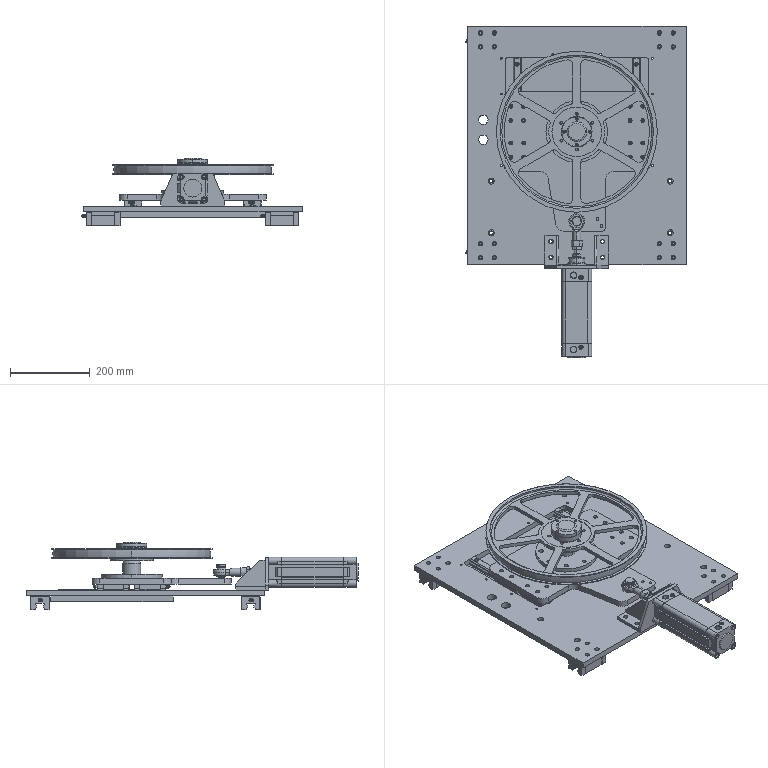Part | SolidWorks | 35 solids | 2701 faces | box 554 x 835 x 169.5 mm | volume 9555082 mm3 | plane 1108 | cylinder 996 | cone 305 | sphere 146 | torus 118 | spline 28 | commonest cylinder face diameters 1 x102 11 x72 6.6 x68 5 x64 0.4 x40 5.5 x40